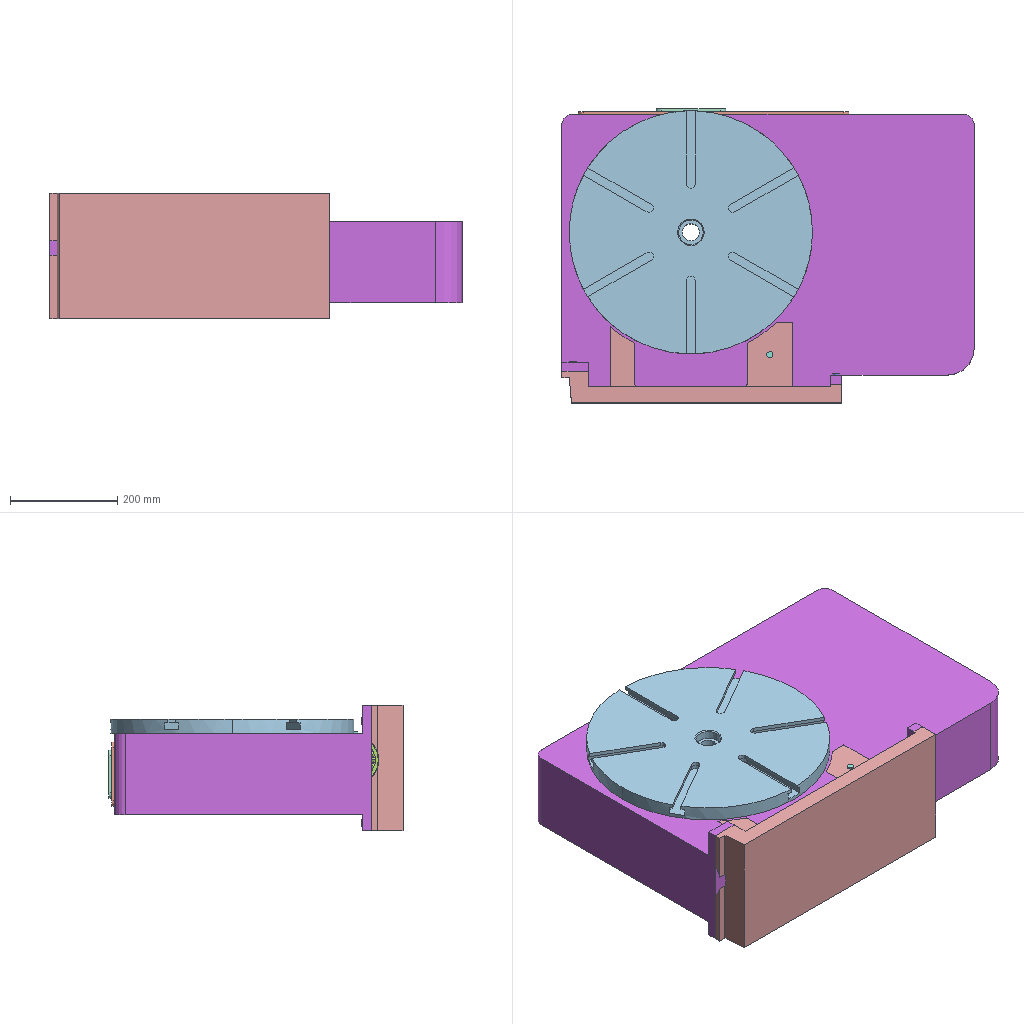Assembly | SolidWorks | 14 different items | 20 placed | box 770 x 549 x 235 mm
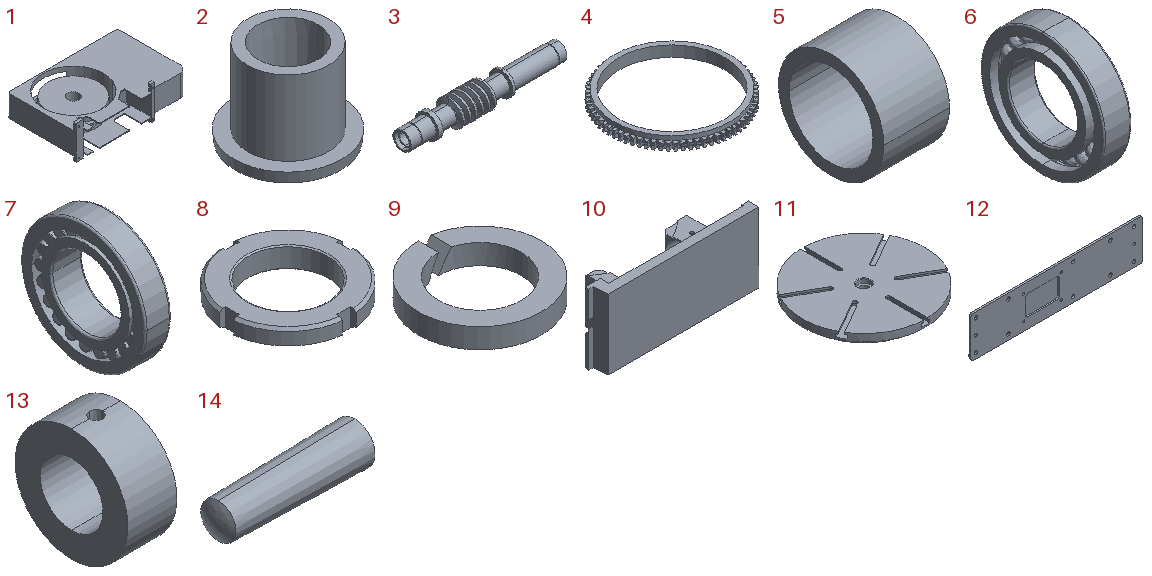Parts list (item | quantity | size | volume | features):
1 | x1 | 770 x 509 x 235 mm | 22102054 mm3 | features ICE 11, Fillet 2, Cut 1, Revolution 1
2 | x1 | 106 x 106 x 84 mm | 252355 mm3 | features Revolution 1
3 | x1 | 425 x 72 x 72 mm | 557558 mm3 | features ICE 13, Chamfer 1, Cut 1, Extrusion 1, Helix 1, RevCut 1, SweepCut 1
4 | x1 | 407.55 x 407.55 x 36 mm | 828010 mm3 | features CirPattern 1, Revolution 1, SweepCut 1
5 | x1 | 39.25 x 63 x 63 mm | 45285 mm3 | features Extrusion 1
6 | x2 | 20 x 90 x 90 mm | 65123 mm3 | features BaseBody 1
7 | x2 | 24.75 x 90 x 90 mm | 73471 mm3 | features BaseBody 1
8 | x2 | 71.554 x 71.554 x 12 mm | 25355 mm3 | features BaseBody 1
9 | x4 | 12.88 x 12.88 x 2.1 mm | 143.98 mm3 | features BaseBody 1
10 | x1 | 523 x 150 x 235 mm | 5356389 mm3 | features Cut 3, ICE 2, Extrusion 1, Fillet 1, HoleWzd 1, RevCut 1
11 | x1 | 454 x 454 x 148.4 mm | 7848995 mm3 | features Cut 2, ICE 2, Chamfer 1, CirPattern 1, Revolution 1
12 | x1 | 505 x 10 x 120 mm | 325188 mm3 | features Fillet 2, ICE 2, Extrusion 1, HoleWzd 1
13 | x1 | 39 x 90 x 90 mm | 169812 mm3 | features Extrusion 1, RevCut 1
14 | x1 | 39.9 x 11.548 x 11.548 mm | 3582 mm3 | features BaseBody 1, Cut 1
Mates (type | each side: item.copy, entity, surface, feature):
Concentric | 3.1 face cylinder Boss-Extrude1 | 6.1 face cylinder Input 1 | 2 times
Concentric | 3.1 face cylinder Boss-Extrude4 | 6.2 face cylinder Input 1
DistanceDim | 3.1 face plane Boss-Extrude5 | 6.2 face plane Input 1
Coincident | 6.2 face plane Input 1 | 6.1 face plane Input 1
Concentric | 10.1 face cone Cut-Revolve1 | 14.1 face cone Input 1
Coincident | 3.1 face plane Boss-Extrude9 | 7.1 face plane Input 1
Concentric | 3.1 face cylinder Boss-Extrude10 | 7.1 face cylinder Input 1
Coincident | 13.1 face plane Boss-Extrude1 | 7.2 face plane Input 1
Concentric | 3.1 face cylinder Boss-Extrude10 | 7.2 face cylinder Input 1
Coincident | 5.1 face plane Boss-Extrude1 | 8.1 face plane Input 1
Concentric | 5.1 face cylinder Boss-Extrude1 | 8.1 face cylinder Input 1
Coincident | 8.1 face plane Input 1 | 8.2 face plane Input 1
Concentric | 8.1 face cylinder Input 1 | 8.2 face cylinder Input 1
Coincident | 1.1 face plane Boss-Extrude1 | 9.1 face plane Input 1
Concentric | 1.1 face cylinder Cut-Extrude2 | 9.1 face cylinder Input 1
Coincident | 1.1 face plane Boss-Extrude1 | 9.2 face plane Input 1
Concentric | 1.1 face cylinder Cut-Extrude2 | 9.2 face cylinder Input 1
Coincident | 1.1 face plane Boss-Extrude10 | 9.3 face plane Input 1
Concentric | 1.1 face cylinder Cut-Extrude2 | 9.3 face cylinder Input 1
Coincident | 1.1 face plane Boss-Extrude10 | 9.4 face plane Input 1
Concentric | 1.1 face cylinder Cut-Extrude2 | 9.4 face cylinder Input 1